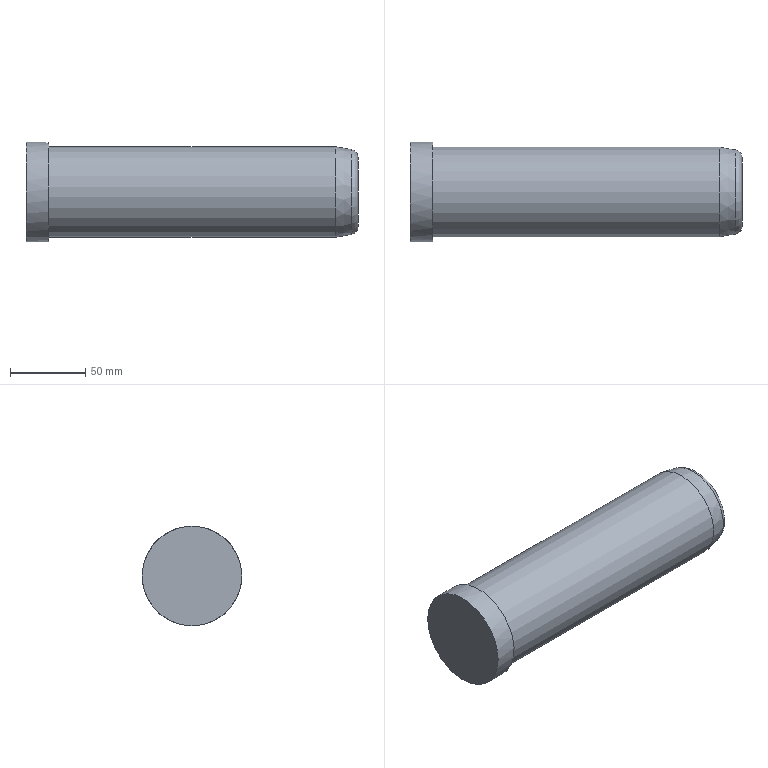Part | STEP file | solid 220 | 1 solid | 7 faces | box 220 x 66 x 66 mm | volume 626724 mm3 | plane 3 | cylinder 2 | cone 1 | torus 1 | commonest cylinder face diameters 60 x1 66 x1